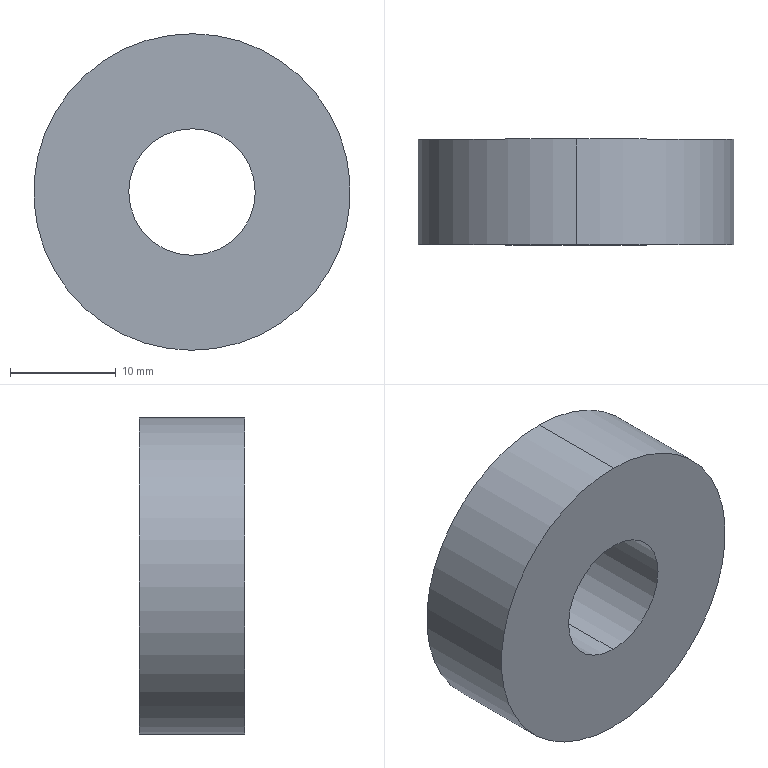Part | NX | features BREP 1 | 1 solid | 6 faces | box 30 x 10 x 30 mm | volume 5938 mm3 | cylinder 4 | plane 2 | commonest cylinder face diameters 12 x2 30 x2
STEP:
#1=CARTESIAN_POINT('',(-0.02557,193.,-6.));
#2=VERTEX_POINT('',#1);
#3=CARTESIAN_POINT('',(0.02557,193.,6.));
#4=VERTEX_POINT('',#3);
#5=CARTESIAN_POINT('',(0.,193.,0.));
#6=DIRECTION('',(0.,-1.,0.));
#7=DIRECTION('',(0.004261,0.,1.));
#8=AXIS2_PLACEMENT_3D('',#5,#6,#7);
#9=CIRCLE('',#8,6.);
#10=EDGE_CURVE('',#2,#4,#9,.T.);
#11=ORIENTED_EDGE('',*,*,#10,.T.);
#12=CARTESIAN_POINT('',(0.02557,203.,6.));
#13=VERTEX_POINT('',#12);
#14=CARTESIAN_POINT('',(0.02557,193.,6.));
#15=DIRECTION('',(0.,1.,0.));
#16=VECTOR('',#15,1000.);
#17=LINE('',#14,#16);
#18=EDGE_CURVE('',#4,#13,#17,.T.);
#19=ORIENTED_EDGE('',*,*,#18,.T.);
#20=CARTESIAN_POINT('',(-0.02557,203.,-6.));
#21=VERTEX_POINT('',#20);
#22=CARTESIAN_POINT('',(0.,203.,0.));
#23=DIRECTION('',(0.,-1.,0.));
#24=DIRECTION('',(0.004261,0.,1.));
#25=AXIS2_PLACEMENT_3D('',#22,#23,#24);
#26=CIRCLE('',#25,6.);
#27=EDGE_CURVE('',#21,#13,#26,.T.);
#28=ORIENTED_EDGE('',*,*,#27,.F.);
#29=CARTESIAN_POINT('',(-0.02557,193.,-6.));
#30=DIRECTION('',(0.,-1.,0.));
#31=VECTOR('',#30,1000.);
#32=LINE('',#29,#31);
#33=EDGE_CURVE('',#21,#2,#32,.T.);
#34=ORIENTED_EDGE('',*,*,#33,.T.);
#35=EDGE_LOOP('',(#11,#19,#28,#34));
#36=FACE_BOUND('',#35,.T.);
#37=CARTESIAN_POINT('',(0.,193.,0.));
#38=DIRECTION('',(0.,1.,0.));
#39=DIRECTION('',(0.004261,0.,1.));
#40=AXIS2_PLACEMENT_3D('',#37,#38,#39);
#41=CYLINDRICAL_SURFACE('',#40,6.);
#42=ADVANCED_FACE('',(#36),#41,.F.);
#43=CARTESIAN_POINT('',(0.06392,193.,15.));
#44=VERTEX_POINT('',#43);
#45=CARTESIAN_POINT('',(-0.06392,193.,-15.));
#46=VERTEX_POINT('',#45);
#47=CARTESIAN_POINT('',(0.,193.,0.));
#48=DIRECTION('',(0.,-1.,0.));
#49=DIRECTION('',(0.004261,0.,1.));
#50=AXIS2_PLACEMENT_3D('',#47,#48,#49);
#51=CIRCLE('',#50,15.);
#52=EDGE_CURVE('',#44,#46,#51,.T.);
#53=ORIENTED_EDGE('',*,*,#52,.F.);
#54=CARTESIAN_POINT('',(0.06392,203.,15.));
#55=VERTEX_POINT('',#54);
#56=CARTESIAN_POINT('',(0.06392,193.,15.));
#57=DIRECTION('',(0.,-1.,0.));
#58=VECTOR('',#57,1000.);
#59=LINE('',#56,#58);
#60=EDGE_CURVE('',#55,#44,#59,.T.);
#61=ORIENTED_EDGE('',*,*,#60,.F.);
#62=CARTESIAN_POINT('',(-0.06392,203.,-15.));
#63=VERTEX_POINT('',#62);
#64=CARTESIAN_POINT('',(0.,203.,0.));
#65=DIRECTION('',(0.,-1.,0.));
#66=DIRECTION('',(0.004261,0.,1.));
#67=AXIS2_PLACEMENT_3D('',#64,#65,#66);
#68=CIRCLE('',#67,15.);
#69=EDGE_CURVE('',#55,#63,#68,.T.);
#70=ORIENTED_EDGE('',*,*,#69,.T.);
#71=CARTESIAN_POINT('',(-0.06392,193.,-15.));
#72=DIRECTION('',(0.,1.,0.));
#73=VECTOR('',#72,1000.);
#74=LINE('',#71,#73);
#75=EDGE_CURVE('',#46,#63,#74,.T.);
#76=ORIENTED_EDGE('',*,*,#75,.F.);
#77=EDGE_LOOP('',(#53,#61,#70,#76));
#78=FACE_BOUND('',#77,.T.);
#79=CARTESIAN_POINT('',(0.,193.,0.));
#80=DIRECTION('',(0.,1.,0.));
#81=DIRECTION('',(0.004261,0.,1.));
#82=AXIS2_PLACEMENT_3D('',#79,#80,#81);
#83=CYLINDRICAL_SURFACE('',#82,15.);
#84=ADVANCED_FACE('',(#78),#83,.T.);
#85=CARTESIAN_POINT('',(0.,193.,0.));
#86=DIRECTION('',(0.,-1.,0.));
#87=DIRECTION('',(0.004261,0.,1.));
#88=AXIS2_PLACEMENT_3D('',#85,#86,#87);
#89=CIRCLE('',#88,15.);
#90=EDGE_CURVE('',#46,#44,#89,.T.);
#91=ORIENTED_EDGE('',*,*,#90,.T.);
#92=ORIENTED_EDGE('',*,*,#52,.T.);
#93=EDGE_LOOP('',(#91,#92));
#94=FACE_BOUND('',#93,.T.);
#95=ORIENTED_EDGE('',*,*,#10,.F.);
#96=CARTESIAN_POINT('',(0.,193.,0.));
#97=DIRECTION('',(0.,-1.,0.));
#98=DIRECTION('',(0.004261,0.,1.));
#99=AXIS2_PLACEMENT_3D('',#96,#97,#98);
#100=CIRCLE('',#99,6.);
#101=EDGE_CURVE('',#4,#2,#100,.T.);
#102=ORIENTED_EDGE('',*,*,#101,.F.);
#103=EDGE_LOOP('',(#95,#102));
#104=FACE_BOUND('',#103,.T.);
#105=CARTESIAN_POINT('',(0.,193.,0.));
#106=DIRECTION('',(0.,-1.,0.));
#107=DIRECTION('',(-0.004261,0.,-1.));
#108=AXIS2_PLACEMENT_3D('',#105,#106,#107);
#109=PLANE('',#108);
#110=ADVANCED_FACE('',(#94,#104),#109,.T.);
#111=CARTESIAN_POINT('',(0.,203.,0.));
#112=DIRECTION('',(0.,-1.,0.));
#113=DIRECTION('',(0.004261,0.,1.));
#114=AXIS2_PLACEMENT_3D('',#111,#112,#113);
#115=CIRCLE('',#114,15.);
#116=EDGE_CURVE('',#63,#55,#115,.T.);
#117=ORIENTED_EDGE('',*,*,#116,.F.);
#118=ORIENTED_EDGE('',*,*,#69,.F.);
#119=EDGE_LOOP('',(#117,#118));
#120=FACE_BOUND('',#119,.T.);
#121=ORIENTED_EDGE('',*,*,#27,.T.);
#122=CARTESIAN_POINT('',(0.,203.,0.));
#123=DIRECTION('',(0.,-1.,0.));
#124=DIRECTION('',(0.004261,0.,1.));
#125=AXIS2_PLACEMENT_3D('',#122,#123,#124);
#126=CIRCLE('',#125,6.);
#127=EDGE_CURVE('',#13,#21,#126,.T.);
#128=ORIENTED_EDGE('',*,*,#127,.T.);
#129=EDGE_LOOP('',(#121,#128));
#130=FACE_BOUND('',#129,.T.);
#131=CARTESIAN_POINT('',(0.,203.,0.));
#132=DIRECTION('',(0.,-1.,0.));
#133=DIRECTION('',(-0.004261,0.,-1.));
#134=AXIS2_PLACEMENT_3D('',#131,#132,#133);
#135=PLANE('',#134);
#136=ADVANCED_FACE('',(#120,#130),#135,.F.);
#137=ORIENTED_EDGE('',*,*,#60,.T.);
#138=ORIENTED_EDGE('',*,*,#90,.F.);
#139=ORIENTED_EDGE('',*,*,#75,.T.);
#140=ORIENTED_EDGE('',*,*,#116,.T.);
#141=EDGE_LOOP('',(#137,#138,#139,#140));
#142=FACE_BOUND('',#141,.T.);
#143=CARTESIAN_POINT('',(0.,193.,0.));
#144=DIRECTION('',(0.,1.,0.));
#145=DIRECTION('',(0.004261,0.,1.));
#146=AXIS2_PLACEMENT_3D('',#143,#144,#145);
#147=CYLINDRICAL_SURFACE('',#146,15.);
#148=ADVANCED_FACE('',(#142),#147,.T.);
#149=ORIENTED_EDGE('',*,*,#18,.F.);
#150=ORIENTED_EDGE('',*,*,#101,.T.);
#151=ORIENTED_EDGE('',*,*,#33,.F.);
#152=ORIENTED_EDGE('',*,*,#127,.F.);
#153=EDGE_LOOP('',(#149,#150,#151,#152));
#154=FACE_BOUND('',#153,.T.);
#155=CARTESIAN_POINT('',(0.,193.,0.));
#156=DIRECTION('',(0.,1.,0.));
#157=DIRECTION('',(0.004261,0.,1.));
#158=AXIS2_PLACEMENT_3D('',#155,#156,#157);
#159=CYLINDRICAL_SURFACE('',#158,6.);
#160=ADVANCED_FACE('',(#154),#159,.F.);
#161=CLOSED_SHELL('',(#42,#84,#110,#136,#148,#160));
#162=MANIFOLD_SOLID_BREP('',#161);
#163=(LENGTH_UNIT()NAMED_UNIT(*)SI_UNIT(.MILLI.,.METRE.));
#164=UNCERTAINTY_MEASURE_WITH_UNIT(LENGTH_MEASURE(0.00001),#163,'','');
#165=(NAMED_UNIT(*)PLANE_ANGLE_UNIT()SI_UNIT($,.RADIAN.));
#166=(NAMED_UNIT(*)SI_UNIT($,.STERADIAN.)SOLID_ANGLE_UNIT());
#167=(GEOMETRIC_REPRESENTATION_CONTEXT(3)GLOBAL_UNCERTAINTY_ASSIGNED_CONTEXT((#164))GLOBAL_UNIT_ASSIGNED_CONTEXT((#163,#165,#166))REPRESENTATION_CONTEXT('',''));
#168=ADVANCED_BREP_SHAPE_REPRESENTATION('',(#162),#167);